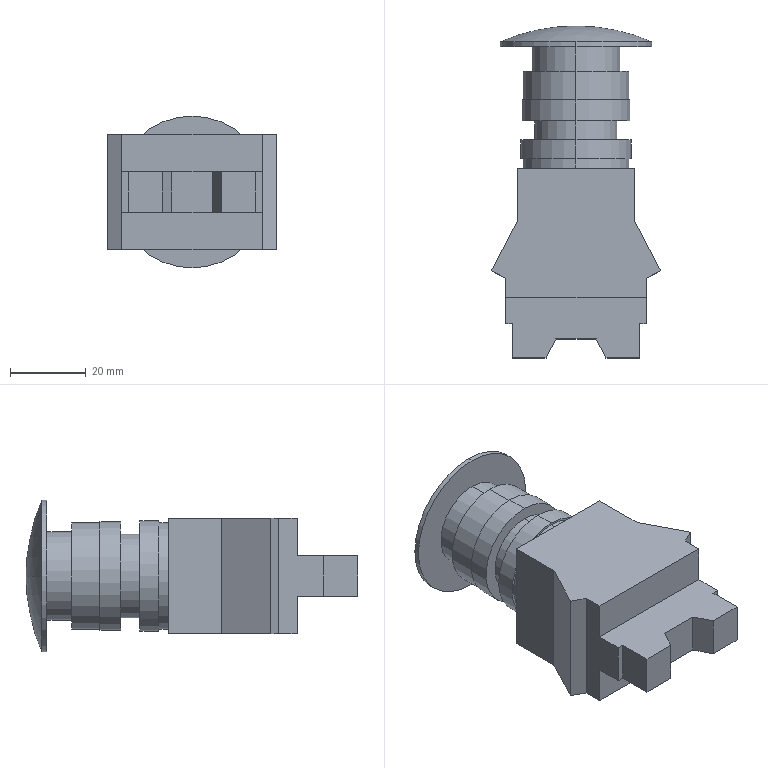Part | STEP file | 1 solid | 46 faces | box 44.567 x 87.5 x 40 mm | volume 63672 mm3 | plane 30 | cylinder 14 | sphere 2 | commonest cylinder face diameters 28 x4 22 x2 23.3 x2 28.65 x2 29.2 x2 40 x2